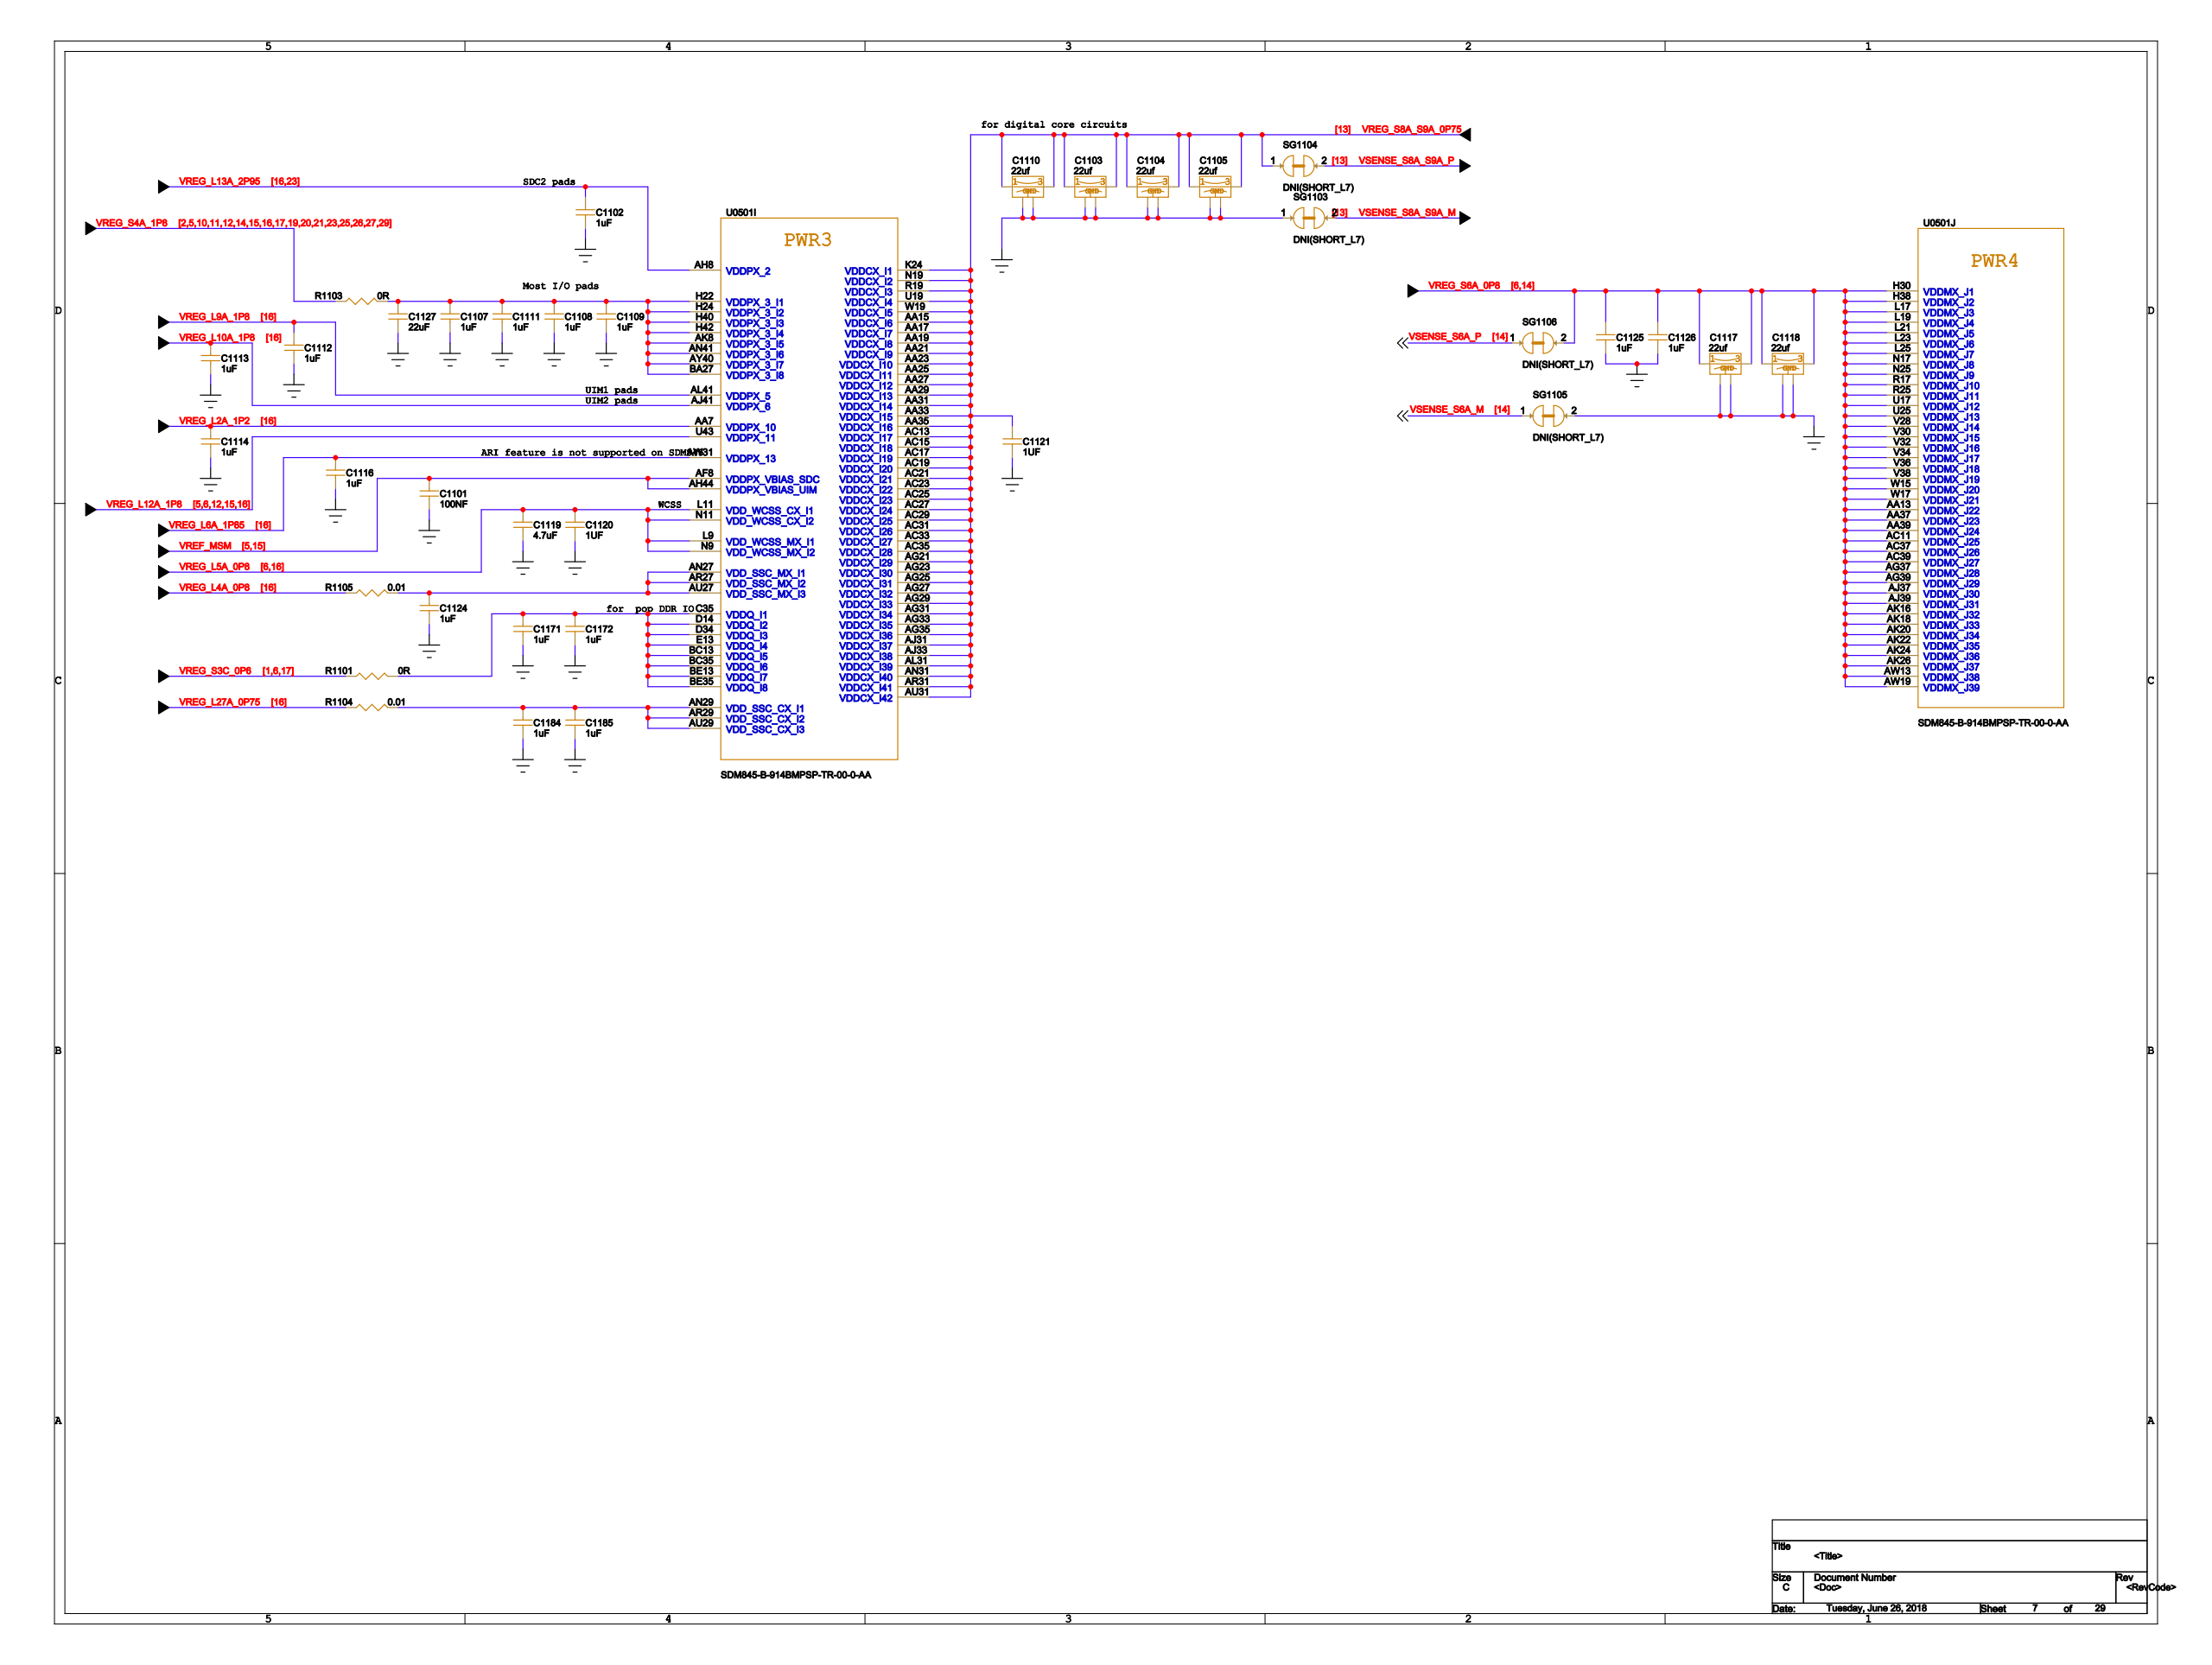Circuit board | Cadence Allegro | 802 parts | 566 nets | one sheet of the schematic
Parts on this sheet (reference | value | footprint):
C1101 | 100NF | C0201
C1102 | 1uF | C0201
C1103 | 22uf | NFMJMPC226R0G3
C1104 | 22uf | NFMJMPC226R0G3
C1105 | 22uf | NFMJMPC226R0G3
C1107 | 1uF | C0201
C1108 | 1uF | C0201
C1109 | 1uF | C0201
C1110 | 22uf | NFMJMPC226R0G3
C1111 | 1uF | C0201
C1112 | 1uF | C0201
C1113 | 1uF | C0201
C1114 | 1uF | C0201
C1116 | 1uF | C0201
C1117 | 22uf | NFMJMPC226R0G3
C1118 | 22uf | NFMJMPC226R0G3
C1119 | 4.7uF | 0402-BIG
C1120 | 1UF | C0402
C1121 | 1UF | C0402
C1124 | 1uF | C0201
C1125 | 1uF | C0201
C1126 | 1uF | C0201
C1127 | 22uF | 0402-BIG
C1171 | 1uF | C0201
C1172 | 1uF | C0201
C1184 | 1uF | C0201
C1185 | 1uF | C0201
R1101 | 0R | R0201
R1103 | 0R | R0603
R1104 | 0.01 | R0603
R1105 | 0.01 | R0603
SG1103 | DNI(SHORT_L7) | SHORT_L7_2REC08X12
SG1104 | DNI(SHORT_L7) | SHORT_L7_2REC08X12
SG1105 | DNI(SHORT_L7) | SHORT_L7_2REC08X12
SG1106 | DNI(SHORT_L7) | SHORT_L7_2REC08X12
U0501 | SDM845-B-914BMPSP-TR-00-0-AA | BGA914_12P4X12P4_0P58_0P35
Nets of these parts (net: part-pin ...):
GND: C1101-2 C1102-2 C1103-2 C1103-4 C1104-2 C1104-4 C1105-2 C1105-4 C1107-2 C1108-2 C1109-2 C1110-2 C1110-4 C1111-2 C1112-2 C1113-2 C1114-2 C1116-2 C1117-2 C1117-4 C1118-2 C1118-4 C1119-2 C1120-2 C1121-2 C1124-2 C1125-2 C1126-2 C1127-2 C1171-2 C1172-2 C1184-2 C1185-2 SG1103-1 SG1105-2
N109892: C1107-1 C1108-1 C1109-1 C1111-1 C1127-1 R1103-2 U0501-AK8 U0501-AN41 U0501-AY40 U0501-BA27 U0501-H22 U0501-H24 U0501-H40 U0501-H42
VREF_MSM: C1101-1 U0501-AF8 U0501-AH44
VREG_S4A_1P8: R1103-1
VREG_S3C_0P6: R1101-1
N113950: C1171-1 C1172-1 R1101-2 U0501-BC13 U0501-BC35 U0501-BE13 U0501-BE35 U0501-C35 U0501-D14 U0501-D34 U0501-E13
VREG_S6A_0P8: C1117-1 C1117-3 C1118-1 C1118-3 C1125-1 C1126-1 SG1106-2 U0501-AA13 U0501-AA37 U0501-AA39 U0501-AC11 U0501-AC37 U0501-AC39 U0501-AG37 U0501-AG39 U0501-AJ37 U0501-AJ39 U0501-AK16 U0501-AK18 U0501-AK20 U0501-AK22 U0501-AK24 U0501-AK26 U0501-AW13 U0501-AW19 U0501-H30 U0501-H38 U0501-L17 U0501-L19 U0501-L21 U0501-L23 U0501-L25 U0501-N17 U0501-N25 U0501-R17 U0501-R25 U0501-U17 U0501-U25 U0501-V28 U0501-V30 U0501-V32 U0501-V34 U0501-V36 U0501-V38 U0501-W15 U0501-W17
VREG_L6A_1P85: C1116-1 U0501-AW31
VREG_L13A_2P95: C1102-1 U0501-AH8
VREG_L12A_1P8: U0501-U43
VREG_L5A_0P8: C1119-1 C1120-1 U0501-L9 U0501-L11 U0501-N9 U0501-N11
VREG_L9A_1P8: C1112-1 U0501-AL41
VREG_L10A_1P8: C1113-1 U0501-AJ41
VREG_L2A_1P2: C1114-1 U0501-AA7
N113537: C1124-1 R1105-2 U0501-AN27 U0501-AR27 U0501-AU27
N114518: C1184-1 C1185-1 R1104-2 U0501-AN29 U0501-AR29 U0501-AU29
VREG_L27A_0P75: R1104-1
VREG_L4A_0P8: R1105-1
VREG_S8A_S9A_0P75: C1103-1 C1103-3 C1104-1 C1104-3 C1105-1 C1105-3 C1110-1 C1110-3 C1121-1 SG1104-1 U0501-AA15 U0501-AA17 U0501-AA19 U0501-AA21 U0501-AA23 U0501-AA25 U0501-AA27 U0501-AA29 U0501-AA31 U0501-AA33 U0501-AA35 U0501-AC13 U0501-AC15 U0501-AC17 U0501-AC19 U0501-AC21 U0501-AC23 U0501-AC25 U0501-AC27 U0501-AC29 U0501-AC31 U0501-AC33 U0501-AC35 U0501-AG21 U0501-AG23 U0501-AG25 U0501-AG27 U0501-AG29 U0501-AG31 U0501-AG33 U0501-AG35 U0501-AJ31 U0501-AJ33 U0501-AL31 U0501-AN31 U0501-AR31 U0501-AU31 U0501-K24 U0501-N19 U0501-R19 U0501-U19 U0501-W19
VSENSE_S8A_S9A_M: SG1103-2
VSENSE_S8A_S9A_P: SG1104-2
VSENSE_S6A_M: SG1105-1
VSENSE_S6A_P: SG1106-1